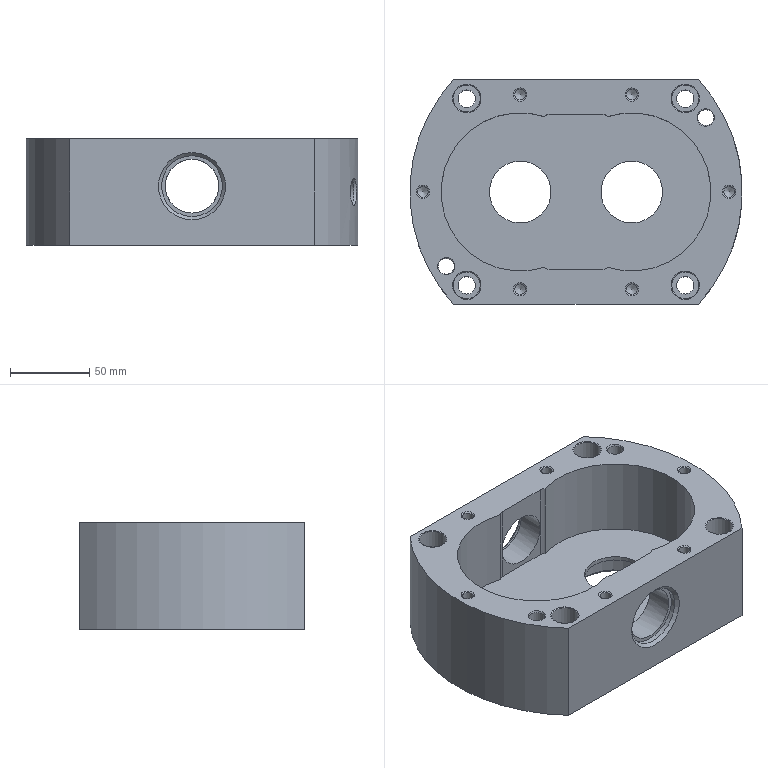NC program | NX | posted with a generic post | part box 210 x 142 x 67.4 mm
Lines 1 to 525 of 22889:
N10 G17 G21 G94 G90
(FLOOR_WALL_COPY_1 , TOOL : D50)
N12 T02 M6
N14 G54
N16 G17 G0 G90 X-143. Y80.997 B0. C0. S1200 M3
N18 G43 Z30. H2
N20 Z12.658
N22 G94 G1 Z9.658 F1000.
N24 X-140.
N26 X140. F2000.
N28 Y45.498
N30 X-140.
N32 Y9.999
N34 X140.
N36 Y-25.501
N38 X-140.
N40 Y-61.
N42 X140.
N44 X143.
N46 Z12.658
N48 G0 Z30.
N50 X-143. Y80.997
N52 Z12.317
N54 G1 Z9.317 F1000.
N56 X-140.
N58 X140. F2000.
N60 Y45.498
N62 X-140.
N64 Y9.999
N66 X140.
N68 Y-25.501
N70 X-140.
N72 Y-61.
N74 X140.
N76 X143.
N78 Z12.317
N80 G0 Z30.
N82 X-143. Y80.997
N84 Z11.976
N86 G1 Z8.976 F1000.
N88 X-140.
N90 X140. F2000.
N92 Y45.498
N94 X-140.
N96 Y9.999
N98 X140.
N100 Y-25.501
N102 X-140.
N104 Y-61.
N106 X140.
N108 X143.
N110 Z11.976
N112 G0 Z30.
N114 X-143. Y80.997
N116 Z11.634
N118 G1 Z8.634 F1000.
N120 X-140.
N122 X140. F2000.
N124 Y45.498
N126 X-140.
N128 Y9.999
N130 X140.
N132 Y-25.501
N134 X-140.
N136 Y-61.
N138 X140.
N140 X143.
N142 Z11.634
N144 G0 Z30.
N146 X-143. Y80.997
N148 Z11.293
N150 G1 Z8.293 F1000.
N152 X-140.
N154 X140. F2000.
N156 Y45.498
N158 X-140.
N160 Y9.999
N162 X140.
N164 Y-25.501
N166 X-140.
N168 Y-61.
N170 X140.
N172 X143.
N174 Z11.293
N176 G0 Z30.
N178 X-143. Y80.997
N180 Z10.951
N182 G1 Z7.951 F1000.
N184 X-140.
N186 X140. F2000.
N188 Y45.498
N190 X-140.
N192 Y9.999
N194 X140.
N196 Y-25.501
N198 X-140.
N200 Y-61.
N202 X140.
N204 X143.
N206 Z10.951
N208 G0 Z30.
N210 X-143. Y80.997
N212 Z10.61
N214 G1 Z7.61 F1000.
N216 X-140.
N218 X140. F2000.
N220 Y45.498
N222 X-140.
N224 Y9.999
N226 X140.
N228 Y-25.501
N230 X-140.
N232 Y-61.
N234 X140.
N236 X143.
N238 Z10.61
N240 G0 Z30.
N242 X-143. Y80.997
N244 Z10.269
N246 G1 Z7.269 F1000.
N248 X-140.
N250 X140. F2000.
N252 Y45.498
N254 X-140.
N256 Y9.999
N258 X140.
N260 Y-25.501
N262 X-140.
N264 Y-61.
N266 X140.
N268 X143.
N270 Z10.269
N272 G0 Z30.
N274 X-143. Y80.997
N276 Z9.927
N278 G1 Z6.927 F1000.
N280 X-140.
N282 X140. F2000.
N284 Y45.498
N286 X-140.
N288 Y9.999
N290 X140.
N292 Y-25.501
N294 X-140.
N296 Y-61.
N298 X140.
N300 X143.
N302 Z9.927
N304 G0 Z30.
N306 X-143. Y80.997
N308 Z9.586
N310 G1 Z6.586 F1000.
N312 X-140.
N314 X140. F2000.
N316 Y45.498
N318 X-140.
N320 Y9.999
N322 X140.
N324 Y-25.501
N326 X-140.
N328 Y-61.
N330 X140.
N332 X143.
N334 Z9.586
N336 G0 Z30.
N338 X-143. Y80.997
N340 Z9.245
N342 G1 Z6.245 F1000.
N344 X-140.
N346 X140. F2000.
N348 Y45.498
N350 X-140.
N352 Y9.999
N354 X140.
N356 Y-25.501
N358 X-140.
N360 Y-61.
N362 X140.
N364 X143.
N366 Z9.245
N368 G0 Z30.
N370 X-143. Y80.997
N372 Z8.903
N374 G1 Z5.903 F1000.
N376 X-140.
N378 X140. F2000.
N380 Y45.498
N382 X-140.
N384 Y9.999
N386 X140.
N388 Y-25.501
N390 X-140.
N392 Y-61.
N394 X140.
N396 X143.
N398 Z8.903
N400 G0 Z30.
N402 X-143. Y80.997
N404 Z8.562
N406 G1 Z5.562 F1000.
N408 X-140.
N410 X140. F2000.
N412 Y45.498
N414 X-140.
N416 Y9.999
N418 X140.
N420 Y-25.501
N422 X-140.
N424 Y-61.
N426 X140.
N428 X143.
N430 Z8.562
N432 G0 Z30.
N434 X-143. Y80.997
N436 Z8.221
N438 G1 Z5.221 F1000.
N440 X-140.
N442 X140. F2000.
N444 Y45.498
N446 X-140.
N448 Y9.999
N450 X140.
N452 Y-25.501
N454 X-140.
N456 Y-61.
N458 X140.
N460 X143.
N462 Z8.221
N464 G0 Z30.
N466 X-143. Y80.997
N468 Z7.879
N470 G1 Z4.879 F1000.
N472 X-140.
N474 X140. F2000.
N476 Y45.498
N478 X-140.
N480 Y9.999
N482 X140.
N484 Y-25.501
N486 X-140.
N488 Y-61.
N490 X140.
N492 X143.
N494 Z7.879
N496 G0 Z30.
N498 X-143. Y80.997
N500 Z7.538
N502 G1 Z4.538 F1000.
N504 X-140.
N506 X140. F2000.
N508 Y45.498
N510 X-140.
N512 Y9.999
N514 X140.
N516 Y-25.501
N518 X-140.
N520 Y-61.
N522 X140.
N524 X143.
N526 Z7.538
N528 G0 Z30.
N530 X-143. Y80.997
N532 Z7.196
N534 G1 Z4.196 F1000.
N536 X-140.
N538 X140. F2000.
N540 Y45.498
N542 X-140.
N544 Y9.999
N546 X140.
N548 Y-25.501
N550 X-140.
N552 Y-61.
N554 X140.
N556 X143.
N558 Z7.196
N560 G0 Z30.
N562 X-143. Y80.997
N564 Z6.855
N566 G1 Z3.855 F1000.
N568 X-140.
N570 X140. F2000.
N572 Y45.498
N574 X-140.
N576 Y9.999
N578 X140.
N580 Y-25.501
N582 X-140.
N584 Y-61.
N586 X140.
N588 X143.
N590 Z6.855
N592 G0 Z30.
N594 X-143. Y80.997
N596 Z6.514
N598 G1 Z3.514 F1000.
N600 X-140.
N602 X140. F2000.
N604 Y45.498
N606 X-140.
N608 Y9.999
N610 X140.
N612 Y-25.501
N614 X-140.
N616 Y-61.
N618 X140.
N620 X143.
N622 Z6.514
N624 G0 Z30.
N626 X-143. Y80.997
N628 Z6.172
N630 G1 Z3.172 F1000.
N632 X-140.
N634 X140. F2000.
N636 Y45.498
N638 X-140.
N640 Y9.999
N642 X140.
N644 Y-25.501
N646 X-140.
N648 Y-61.
N650 X140.
N652 X143.
N654 Z6.172
N656 G0 Z30.
N658 X-143. Y80.997
N660 Z5.831
N662 G1 Z2.831 F1000.
N664 X-140.
N666 X140. F2000.
N668 Y45.498
N670 X-140.
N672 Y9.999
N674 X140.
N676 Y-25.501
N678 X-140.
N680 Y-61.
N682 X140.
N684 X143.
N686 Z5.831
N688 G0 Z30.
N690 X-143. Y80.997
N692 Z5.49
N694 G1 Z2.49 F1000.
N696 X-140.
N698 X140. F2000.
N700 Y45.498
N702 X-140.
N704 Y9.999
N706 X140.
N708 Y-25.501
N710 X-140.
N712 Y-61.
N714 X140.
N716 X143.
N718 Z5.49
N720 G0 Z30.
N722 X-143. Y80.997
N724 Z5.148
N726 G1 Z2.148 F1000.
N728 X-140.
N730 X140. F2000.
N732 Y45.498
N734 X-140.
N736 Y9.999
N738 X140.
N740 Y-25.501
N742 X-140.
N744 Y-61.
N746 X140.
N748 X143.
N750 Z5.148
N752 G0 Z30.
N754 X-143. Y80.997
N756 Z4.807
N758 G1 Z1.807 F1000.
N760 X-140.
N762 X140. F2000.
N764 Y45.498
N766 X-140.
N768 Y9.999
N770 X140.
N772 Y-25.501
N774 X-140.
N776 Y-61.
N778 X140.
N780 X143.
N782 Z4.807
N784 G0 Z30.
N786 X-143. Y80.997
N788 Z4.465
N790 G1 Z1.465 F1000.
N792 X-140.
N794 X140. F2000.
N796 Y45.498
N798 X-140.
N800 Y9.999
N802 X140.
N804 Y-25.501
N806 X-140.
N808 Y-61.
N810 X140.
N812 X143.
N814 Z4.465
N816 G0 Z30.
N818 X-143. Y80.997
N820 Z4.124
N822 G1 Z1.124 F1000.
N824 X-140.
N826 X140. F2000.
N828 Y45.498
N830 X-140.
N832 Y9.999
N834 X140.
N836 Y-25.501
N838 X-140.
N840 Y-61.
N842 X140.
N844 X143.
N846 Z4.124
N848 G0 Z30.
N850 X-143. Y80.997
N852 Z3.783
N854 G1 Z0.783 F1000.
N856 X-140.
N858 X140. F2000.
N860 Y45.498
N862 X-140.
N864 Y9.999
N866 X140.
N868 Y-25.501
N870 X-140.
N872 Y-61.
N874 X140.
N876 X143.
N878 Z3.783
N880 G0 Z30.
N882 X-143. Y80.997
N884 Z3.441
N886 G1 Z0.441 F1000.
N888 X-140.
N890 X140. F2000.
N892 Y45.498
N894 X-140.
N896 Y9.999
N898 X140.
N900 Y-25.501
N902 X-140.
N904 Y-61.
N906 X140.
N908 X143.
N910 Z3.441
N912 G0 Z30.
N914 X-143. Y80.997
N916 Z3.1
N918 G1 Z0.1 F1000.
N920 X-140.
N922 X140. F2000.
N924 Y45.498
N926 X-140.
N928 Y9.999
N930 X140.
N932 Y-25.501
N934 X-140.
N936 Y-61.
N938 X140.
N940 X143.
N942 Z3.1
N944 G0 Z30.
(FLOOR_WALL_COPY_COPY , TOOL : D50)
N946 X-143. Y80.997 S2500
N948 Z3.
N950 G1 Z0. F1000.
N952 X-140.
N954 X140.
N956 Y45.498
N958 X-140.
N960 Y9.999
N962 X140.
N964 Y-25.501
N966 X-140.
N968 Y-61.
N970 X140.
N972 X143.
N974 Z3.
N976 G0 Z30.
N978 M5
(DRILLING_COPY_1 , TOOL : ZXZ)
N980 T01 M6
N982 G54
N984 G17 G0 G90 X96.75 Y0. B0. C0. S5000 M3
N986 G43 Z30. H1
N988 G94 G81 G98 Z-1. F250. R3.
N990 X35.25 Y-61.5
N992 X-35.25
N994 X-96.75 Y0.
N996 X-35.25 Y61.5
N998 X35.25
N1000 G80
N1002 G0 X35.25 Y61.5 Z30.
N1004 M5
(DRILLING_COPY_1_COPY , TOOL : 6.8ZT)
N1006 T16 M6
N1008 G54
N1010 G17 G0 G90 X96.75 Y0. B0. C0. S2000 M3
N1012 G43 Z30. H16
N1014 G94 G83 G98 Z-22.043 F200. Q2. R3.
N1016 X35.25 Y-61.5
N1018 X-35.25
N1020 X-96.75 Y0.
N1022 X-35.25 Y61.5
N1024 X35.25
N1026 G80
N1028 G0 X35.25 Y61.5 Z30.
N1030 M5